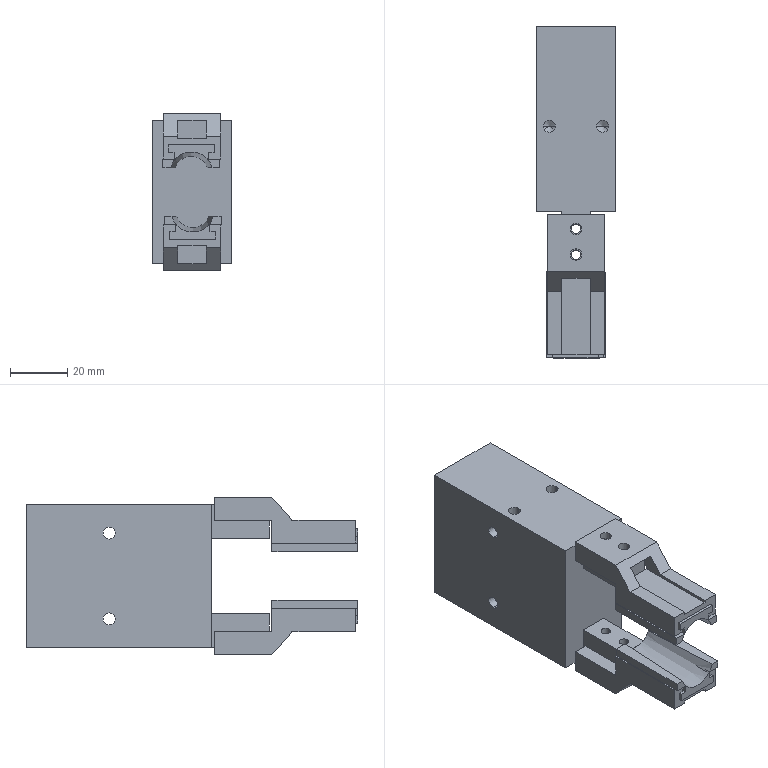Part | 5 solids | 388 faces | box 27.6 x 115.8 x 55 mm | volume 107227 mm3 | plane 255 | spline 103 | cylinder 24 | cone 6 | commonest cylinder face diameters 3.3 x8 4 x8 4.2 x8